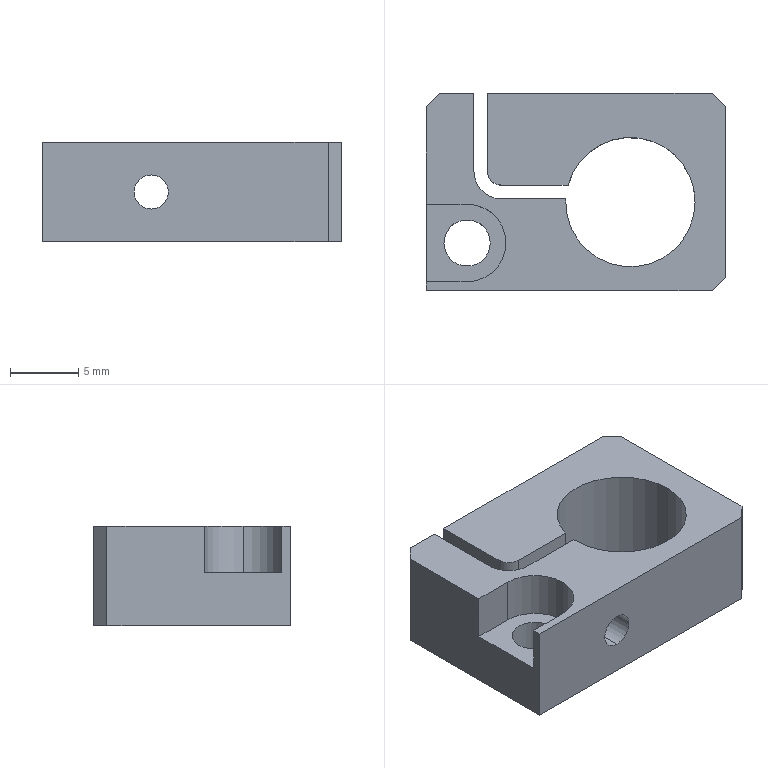Part | SolidWorks | features ICE 4, HoleWzd 3, Fillet 2, Chamfer 1, Extrusion 1 | 1 solid | 33 faces | box 22 x 14.5 x 7.3 mm | volume 1409 mm3 | plane 18 | cylinder 15 | commonest cylinder face diameters 3.4 x4 9.5 x3 2.5 x2 5.7 x2 6 x2 2 x1
STEP:
#1=CARTESIAN_POINT('',(-5.15,-3.75,3.9));
#2=VERTEX_POINT('',#1);
#3=CARTESIAN_POINT('',(-8.,-0.9,3.9));
#4=VERTEX_POINT('',#3);
#5=CARTESIAN_POINT('',(-8.,-3.75,3.9));
#6=DIRECTION('',(0.,0.,1.));
#7=DIRECTION('',(1.,0.,0.));
#8=AXIS2_PLACEMENT_3D('',#5,#6,#7);
#9=CIRCLE('',#8,2.85);
#10=EDGE_CURVE('',#2,#4,#9,.T.);
#11=ORIENTED_EDGE('',*,*,#10,.F.);
#12=CARTESIAN_POINT('',(-5.15,-3.75,7.3));
#13=VERTEX_POINT('',#12);
#14=CARTESIAN_POINT('',(-5.15,-3.75,3.9));
#15=DIRECTION('',(0.,0.,1.));
#16=VECTOR('',#15,1000.);
#17=LINE('',#14,#16);
#18=EDGE_CURVE('',#2,#13,#17,.T.);
#19=ORIENTED_EDGE('',*,*,#18,.T.);
#20=CARTESIAN_POINT('',(-8.,-0.9,7.3));
#21=VERTEX_POINT('',#20);
#22=CARTESIAN_POINT('',(-8.,-3.75,7.3));
#23=DIRECTION('',(0.,0.,1.));
#24=DIRECTION('',(1.,0.,0.));
#25=AXIS2_PLACEMENT_3D('',#22,#23,#24);
#26=CIRCLE('',#25,2.85);
#27=EDGE_CURVE('',#13,#21,#26,.T.);
#28=ORIENTED_EDGE('',*,*,#27,.T.);
#29=CARTESIAN_POINT('',(-8.,-0.9,3.9));
#30=DIRECTION('',(0.,0.,1.));
#31=VECTOR('',#30,1000.);
#32=LINE('',#29,#31);
#33=EDGE_CURVE('',#4,#21,#32,.T.);
#34=ORIENTED_EDGE('',*,*,#33,.F.);
#35=EDGE_LOOP('',(#11,#19,#28,#34));
#36=FACE_OUTER_BOUND('',#35,.T.);
#37=CARTESIAN_POINT('',(-8.,-3.75,3.9));
#38=DIRECTION('',(0.,0.,1.));
#39=DIRECTION('',(1.,0.,0.));
#40=AXIS2_PLACEMENT_3D('',#37,#38,#39);
#41=CYLINDRICAL_SURFACE('',#40,2.85);
#42=ADVANCED_FACE('',(#36),#41,.F.);
#43=CARTESIAN_POINT('',(-3.,3.85,0.65));
#44=VERTEX_POINT('',#43);
#45=CARTESIAN_POINT('',(-3.,3.85,6.65));
#46=VERTEX_POINT('',#45);
#47=CARTESIAN_POINT('',(-3.,3.85,3.65));
#48=DIRECTION('',(0.,1.,0.));
#49=DIRECTION('',(0.,0.,1.));
#50=AXIS2_PLACEMENT_3D('',#47,#48,#49);
#51=CIRCLE('',#50,3.);
#52=EDGE_CURVE('',#44,#46,#51,.T.);
#53=ORIENTED_EDGE('',*,*,#52,.F.);
#54=CARTESIAN_POINT('',(-3.,7.25,0.65));
#55=VERTEX_POINT('',#54);
#56=CARTESIAN_POINT('',(-3.,7.25,0.65));
#57=DIRECTION('',(0.,1.,0.));
#58=VECTOR('',#57,1000.);
#59=LINE('',#56,#58);
#60=EDGE_CURVE('',#44,#55,#59,.T.);
#61=ORIENTED_EDGE('',*,*,#60,.T.);
#62=CARTESIAN_POINT('',(-3.,7.25,6.65));
#63=VERTEX_POINT('',#62);
#64=CARTESIAN_POINT('',(-3.,7.25,3.65));
#65=DIRECTION('',(0.,1.,0.));
#66=DIRECTION('',(0.,0.,1.));
#67=AXIS2_PLACEMENT_3D('',#64,#65,#66);
#68=CIRCLE('',#67,3.);
#69=EDGE_CURVE('',#55,#63,#68,.T.);
#70=ORIENTED_EDGE('',*,*,#69,.T.);
#71=CARTESIAN_POINT('',(-3.,7.25,6.65));
#72=DIRECTION('',(0.,1.,0.));
#73=VECTOR('',#72,1000.);
#74=LINE('',#71,#73);
#75=EDGE_CURVE('',#46,#63,#74,.T.);
#76=ORIENTED_EDGE('',*,*,#75,.F.);
#77=EDGE_LOOP('',(#53,#61,#70,#76));
#78=FACE_OUTER_BOUND('',#77,.T.);
#79=CARTESIAN_POINT('',(-3.,7.25,3.65));
#80=DIRECTION('',(0.,1.,0.));
#81=DIRECTION('',(0.,0.,1.));
#82=AXIS2_PLACEMENT_3D('',#79,#80,#81);
#83=CYLINDRICAL_SURFACE('',#82,3.);
#84=ADVANCED_FACE('',(#78),#83,.F.);
#85=CARTESIAN_POINT('',(-3.,0.5,1.95));
#86=VERTEX_POINT('',#85);
#87=CARTESIAN_POINT('',(-3.,0.5,5.35));
#88=VERTEX_POINT('',#87);
#89=CARTESIAN_POINT('',(-3.,0.5,3.65));
#90=DIRECTION('',(0.,1.,0.));
#91=DIRECTION('',(0.,0.,1.));
#92=AXIS2_PLACEMENT_3D('',#89,#90,#91);
#93=CIRCLE('',#92,1.7);
#94=EDGE_CURVE('',#86,#88,#93,.T.);
#95=ORIENTED_EDGE('',*,*,#94,.F.);
#96=CARTESIAN_POINT('',(-3.,3.85,1.95));
#97=VERTEX_POINT('',#96);
#98=CARTESIAN_POINT('',(-3.,7.25,1.95));
#99=DIRECTION('',(0.,1.,0.));
#100=VECTOR('',#99,1000.);
#101=LINE('',#98,#100);
#102=EDGE_CURVE('',#86,#97,#101,.T.);
#103=ORIENTED_EDGE('',*,*,#102,.T.);
#104=CARTESIAN_POINT('',(-3.,3.85,5.35));
#105=VERTEX_POINT('',#104);
#106=CARTESIAN_POINT('',(-3.,3.85,3.65));
#107=DIRECTION('',(0.,1.,0.));
#108=DIRECTION('',(0.,0.,1.));
#109=AXIS2_PLACEMENT_3D('',#106,#107,#108);
#110=CIRCLE('',#109,1.7);
#111=EDGE_CURVE('',#97,#105,#110,.T.);
#112=ORIENTED_EDGE('',*,*,#111,.T.);
#113=CARTESIAN_POINT('',(-3.,7.25,5.35));
#114=DIRECTION('',(0.,1.,0.));
#115=VECTOR('',#114,1000.);
#116=LINE('',#113,#115);
#117=EDGE_CURVE('',#88,#105,#116,.T.);
#118=ORIENTED_EDGE('',*,*,#117,.F.);
#119=EDGE_LOOP('',(#95,#103,#112,#118));
#120=FACE_OUTER_BOUND('',#119,.T.);
#121=CARTESIAN_POINT('',(-3.,7.25,3.65));
#122=DIRECTION('',(0.,1.,0.));
#123=DIRECTION('',(0.,0.,1.));
#124=AXIS2_PLACEMENT_3D('',#121,#122,#123);
#125=CYLINDRICAL_SURFACE('',#124,1.7);
#126=ADVANCED_FACE('',(#120),#125,.F.);
#127=CARTESIAN_POINT('',(-3.,-7.25,2.4));
#128=VERTEX_POINT('',#127);
#129=CARTESIAN_POINT('',(-3.,-7.25,4.9));
#130=VERTEX_POINT('',#129);
#131=CARTESIAN_POINT('',(-3.,-7.25,3.65));
#132=DIRECTION('',(0.,1.,0.));
#133=DIRECTION('',(0.,0.,1.));
#134=AXIS2_PLACEMENT_3D('',#131,#132,#133);
#135=CIRCLE('',#134,1.25);
#136=EDGE_CURVE('',#128,#130,#135,.T.);
#137=ORIENTED_EDGE('',*,*,#136,.F.);
#138=CARTESIAN_POINT('',(-3.,-0.5,2.4));
#139=VERTEX_POINT('',#138);
#140=CARTESIAN_POINT('',(-3.,-0.5,2.4));
#141=DIRECTION('',(0.,1.,0.));
#142=VECTOR('',#141,1000.);
#143=LINE('',#140,#142);
#144=EDGE_CURVE('',#128,#139,#143,.T.);
#145=ORIENTED_EDGE('',*,*,#144,.T.);
#146=CARTESIAN_POINT('',(-3.,-0.5,4.9));
#147=VERTEX_POINT('',#146);
#148=CARTESIAN_POINT('',(-3.,-0.5,3.65));
#149=DIRECTION('',(0.,1.,0.));
#150=DIRECTION('',(0.,0.,1.));
#151=AXIS2_PLACEMENT_3D('',#148,#149,#150);
#152=CIRCLE('',#151,1.25);
#153=EDGE_CURVE('',#139,#147,#152,.T.);
#154=ORIENTED_EDGE('',*,*,#153,.T.);
#155=CARTESIAN_POINT('',(-3.,-0.5,4.9));
#156=DIRECTION('',(0.,1.,0.));
#157=VECTOR('',#156,1000.);
#158=LINE('',#155,#157);
#159=EDGE_CURVE('',#130,#147,#158,.T.);
#160=ORIENTED_EDGE('',*,*,#159,.F.);
#161=EDGE_LOOP('',(#137,#145,#154,#160));
#162=FACE_OUTER_BOUND('',#161,.T.);
#163=CARTESIAN_POINT('',(-3.,-0.5,3.65));
#164=DIRECTION('',(0.,1.,0.));
#165=DIRECTION('',(0.,0.,1.));
#166=AXIS2_PLACEMENT_3D('',#163,#164,#165);
#167=CYLINDRICAL_SURFACE('',#166,1.25);
#168=ADVANCED_FACE('',(#162),#167,.F.);
#169=CARTESIAN_POINT('',(-0.75,-0.75,0.));
#170=VERTEX_POINT('',#169);
#171=CARTESIAN_POINT('',(8.75,-0.75,0.));
#172=VERTEX_POINT('',#171);
#173=CARTESIAN_POINT('',(4.,-0.75,0.));
#174=DIRECTION('',(0.,0.,1.));
#175=DIRECTION('',(1.,0.,0.));
#176=AXIS2_PLACEMENT_3D('',#173,#174,#175);
#177=CIRCLE('',#176,4.75);
#178=EDGE_CURVE('',#170,#172,#177,.T.);
#179=ORIENTED_EDGE('',*,*,#178,.F.);
#180=CARTESIAN_POINT('',(-0.75,-0.75,7.3));
#181=VERTEX_POINT('',#180);
#182=CARTESIAN_POINT('',(-0.75,-0.75,0.));
#183=DIRECTION('',(0.,0.,1.));
#184=VECTOR('',#183,1000.);
#185=LINE('',#182,#184);
#186=EDGE_CURVE('',#170,#181,#185,.T.);
#187=ORIENTED_EDGE('',*,*,#186,.T.);
#188=CARTESIAN_POINT('',(8.75,-0.75,7.3));
#189=VERTEX_POINT('',#188);
#190=CARTESIAN_POINT('',(4.,-0.75,7.3));
#191=DIRECTION('',(0.,0.,1.));
#192=DIRECTION('',(1.,0.,0.));
#193=AXIS2_PLACEMENT_3D('',#190,#191,#192);
#194=CIRCLE('',#193,4.75);
#195=EDGE_CURVE('',#181,#189,#194,.T.);
#196=ORIENTED_EDGE('',*,*,#195,.T.);
#197=CARTESIAN_POINT('',(8.75,-0.75,0.));
#198=DIRECTION('',(0.,0.,1.));
#199=VECTOR('',#198,1000.);
#200=LINE('',#197,#199);
#201=EDGE_CURVE('',#172,#189,#200,.T.);
#202=ORIENTED_EDGE('',*,*,#201,.F.);
#203=EDGE_LOOP('',(#179,#187,#196,#202));
#204=FACE_OUTER_BOUND('',#203,.T.);
#205=CARTESIAN_POINT('',(4.,-0.75,0.));
#206=DIRECTION('',(0.,0.,1.));
#207=DIRECTION('',(1.,0.,0.));
#208=AXIS2_PLACEMENT_3D('',#205,#206,#207);
#209=CYLINDRICAL_SURFACE('',#208,4.75);
#210=ADVANCED_FACE('',(#204),#209,.F.);
#211=CARTESIAN_POINT('',(-0.5826,0.5,0.));
#212=VERTEX_POINT('',#211);
#213=CARTESIAN_POINT('',(4.,-0.75,0.));
#214=DIRECTION('',(0.,0.,1.));
#215=DIRECTION('',(1.,0.,0.));
#216=AXIS2_PLACEMENT_3D('',#213,#214,#215);
#217=CIRCLE('',#216,4.75);
#218=EDGE_CURVE('',#172,#212,#217,.T.);
#219=ORIENTED_EDGE('',*,*,#218,.F.);
#220=ORIENTED_EDGE('',*,*,#201,.T.);
#221=CARTESIAN_POINT('',(-0.5826,0.5,7.3));
#222=VERTEX_POINT('',#221);
#223=CARTESIAN_POINT('',(4.,-0.75,7.3));
#224=DIRECTION('',(0.,0.,1.));
#225=DIRECTION('',(1.,0.,0.));
#226=AXIS2_PLACEMENT_3D('',#223,#224,#225);
#227=CIRCLE('',#226,4.75);
#228=EDGE_CURVE('',#189,#222,#227,.T.);
#229=ORIENTED_EDGE('',*,*,#228,.T.);
#230=CARTESIAN_POINT('',(-0.5826,0.5,0.));
#231=DIRECTION('',(0.,0.,-1.));
#232=VECTOR('',#231,1000.);
#233=LINE('',#230,#232);
#234=EDGE_CURVE('',#222,#212,#233,.T.);
#235=ORIENTED_EDGE('',*,*,#234,.T.);
#236=EDGE_LOOP('',(#219,#220,#229,#235));
#237=FACE_OUTER_BOUND('',#236,.T.);
#238=CARTESIAN_POINT('',(4.,-0.75,0.));
#239=DIRECTION('',(0.,0.,1.));
#240=DIRECTION('',(1.,0.,0.));
#241=AXIS2_PLACEMENT_3D('',#238,#239,#240);
#242=CYLINDRICAL_SURFACE('',#241,4.75);
#243=ADVANCED_FACE('',(#237),#242,.F.);
#244=CARTESIAN_POINT('',(-9.7,-3.75,0.));
#245=VERTEX_POINT('',#244);
#246=CARTESIAN_POINT('',(-6.3,-3.75,0.));
#247=VERTEX_POINT('',#246);
#248=CARTESIAN_POINT('',(-8.,-3.75,0.));
#249=DIRECTION('',(0.,0.,1.));
#250=DIRECTION('',(1.,0.,0.));
#251=AXIS2_PLACEMENT_3D('',#248,#249,#250);
#252=CIRCLE('',#251,1.7);
#253=EDGE_CURVE('',#245,#247,#252,.T.);
#254=ORIENTED_EDGE('',*,*,#253,.F.);
#255=CARTESIAN_POINT('',(-9.7,-3.75,3.9));
#256=VERTEX_POINT('',#255);
#257=CARTESIAN_POINT('',(-9.7,-3.75,7.3));
#258=DIRECTION('',(0.,0.,1.));
#259=VECTOR('',#258,1000.);
#260=LINE('',#257,#259);
#261=EDGE_CURVE('',#245,#256,#260,.T.);
#262=ORIENTED_EDGE('',*,*,#261,.T.);
#263=CARTESIAN_POINT('',(-6.3,-3.75,3.9));
#264=VERTEX_POINT('',#263);
#265=CARTESIAN_POINT('',(-8.,-3.75,3.9));
#266=DIRECTION('',(0.,0.,-1.));
#267=DIRECTION('',(1.,0.,0.));
#268=AXIS2_PLACEMENT_3D('',#265,#266,#267);
#269=CIRCLE('',#268,1.7);
#270=EDGE_CURVE('',#264,#256,#269,.T.);
#271=ORIENTED_EDGE('',*,*,#270,.F.);
#272=CARTESIAN_POINT('',(-6.3,-3.75,7.3));
#273=DIRECTION('',(0.,0.,1.));
#274=VECTOR('',#273,1000.);
#275=LINE('',#272,#274);
#276=EDGE_CURVE('',#247,#264,#275,.T.);
#277=ORIENTED_EDGE('',*,*,#276,.F.);
#278=EDGE_LOOP('',(#254,#262,#271,#277));
#279=FACE_OUTER_BOUND('',#278,.T.);
#280=CARTESIAN_POINT('',(-8.,-3.75,7.3));
#281=DIRECTION('',(0.,0.,1.));
#282=DIRECTION('',(1.,0.,0.));
#283=AXIS2_PLACEMENT_3D('',#280,#281,#282);
#284=CYLINDRICAL_SURFACE('',#283,1.7);
#285=ADVANCED_FACE('',(#279),#284,.F.);
#286=ORIENTED_EDGE('',*,*,#261,.F.);
#287=CARTESIAN_POINT('',(-8.,-3.75,0.));
#288=DIRECTION('',(0.,0.,1.));
#289=DIRECTION('',(1.,0.,0.));
#290=AXIS2_PLACEMENT_3D('',#287,#288,#289);
#291=CIRCLE('',#290,1.7);
#292=EDGE_CURVE('',#247,#245,#291,.T.);
#293=ORIENTED_EDGE('',*,*,#292,.F.);
#294=ORIENTED_EDGE('',*,*,#276,.T.);
#295=CARTESIAN_POINT('',(-8.,-3.75,3.9));
#296=DIRECTION('',(0.,0.,-1.));
#297=DIRECTION('',(1.,0.,0.));
#298=AXIS2_PLACEMENT_3D('',#295,#296,#297);
#299=CIRCLE('',#298,1.7);
#300=EDGE_CURVE('',#256,#264,#299,.T.);
#301=ORIENTED_EDGE('',*,*,#300,.F.);
#302=EDGE_LOOP('',(#286,#293,#294,#301));
#303=FACE_OUTER_BOUND('',#302,.T.);
#304=CARTESIAN_POINT('',(-8.,-3.75,7.3));
#305=DIRECTION('',(0.,0.,1.));
#306=DIRECTION('',(1.,0.,0.));
#307=AXIS2_PLACEMENT_3D('',#304,#305,#306);
#308=CYLINDRICAL_SURFACE('',#307,1.7);
#309=ADVANCED_FACE('',(#303),#308,.F.);
#310=CARTESIAN_POINT('',(-7.5,7.25,0.));
#311=VERTEX_POINT('',#310);
#312=CARTESIAN_POINT('',(-10.,7.25,0.));
#313=VERTEX_POINT('',#312);
#314=CARTESIAN_POINT('',(-11.,7.25,0.));
#315=DIRECTION('',(-1.,0.,0.));
#316=VECTOR('',#315,1000.);
#317=LINE('',#314,#316);
#318=EDGE_CURVE('',#311,#313,#317,.T.);
#319=ORIENTED_EDGE('',*,*,#318,.T.);
#320=CARTESIAN_POINT('',(-10.,7.25,7.3));
#321=VERTEX_POINT('',#320);
#322=CARTESIAN_POINT('',(-10.,7.25,7.3));
#323=DIRECTION('',(0.,0.,1.));
#324=VECTOR('',#323,1000.);
#325=LINE('',#322,#324);
#326=EDGE_CURVE('',#313,#321,#325,.T.);
#327=ORIENTED_EDGE('',*,*,#326,.T.);
#328=CARTESIAN_POINT('',(-7.5,7.25,7.3));
#329=VERTEX_POINT('',#328);
#330=CARTESIAN_POINT('',(-11.,7.25,7.3));
#331=DIRECTION('',(-1.,0.,0.));
#332=VECTOR('',#331,1000.);
#333=LINE('',#330,#332);
#334=EDGE_CURVE('',#329,#321,#333,.T.);
#335=ORIENTED_EDGE('',*,*,#334,.F.);
#336=CARTESIAN_POINT('',(-7.5,7.25,-9.7));
#337=DIRECTION('',(0.,0.,1.));
#338=VECTOR('',#337,1000.);
#339=LINE('',#336,#338);
#340=EDGE_CURVE('',#311,#329,#339,.T.);
#341=ORIENTED_EDGE('',*,*,#340,.F.);
#342=EDGE_LOOP('',(#319,#327,#335,#341));
#343=FACE_OUTER_BOUND('',#342,.T.);
#344=CARTESIAN_POINT('',(-11.,7.25,7.3));
#345=DIRECTION('',(0.,-1.,0.));
#346=DIRECTION('',(0.,0.,-1.));
#347=AXIS2_PLACEMENT_3D('',#344,#345,#346);
#348=PLANE('',#347);
#349=ADVANCED_FACE('',(#343),#348,.F.);
#350=CARTESIAN_POINT('',(11.,-6.25,7.3));
#351=VERTEX_POINT('',#350);
#352=CARTESIAN_POINT('',(11.,6.25,7.3));
#353=VERTEX_POINT('',#352);
#354=CARTESIAN_POINT('',(11.,-7.25,7.3));
#355=DIRECTION('',(0.,1.,0.));
#356=VECTOR('',#355,1000.);
#357=LINE('',#354,#356);
#358=EDGE_CURVE('',#351,#353,#357,.T.);
#359=ORIENTED_EDGE('',*,*,#358,.F.);
#360=CARTESIAN_POINT('',(11.,-6.25,0.));
#361=VERTEX_POINT('',#360);
#362=CARTESIAN_POINT('',(11.,-6.25,7.3));
#363=DIRECTION('',(0.,0.,-1.));
#364=VECTOR('',#363,1000.);
#365=LINE('',#362,#364);
#366=EDGE_CURVE('',#351,#361,#365,.T.);
#367=ORIENTED_EDGE('',*,*,#366,.T.);
#368=CARTESIAN_POINT('',(11.,6.25,0.));
#369=VERTEX_POINT('',#368);
#370=CARTESIAN_POINT('',(11.,-7.25,0.));
#371=DIRECTION('',(0.,1.,0.));
#372=VECTOR('',#371,1000.);
#373=LINE('',#370,#372);
#374=EDGE_CURVE('',#361,#369,#373,.T.);
#375=ORIENTED_EDGE('',*,*,#374,.T.);
#376=CARTESIAN_POINT('',(11.,6.25,7.3));
#377=DIRECTION('',(0.,0.,1.));
#378=VECTOR('',#377,1000.);
#379=LINE('',#376,#378);
#380=EDGE_CURVE('',#369,#353,#379,.T.);
#381=ORIENTED_EDGE('',*,*,#380,.T.);
#382=EDGE_LOOP('',(#359,#367,#375,#381));
#383=FACE_OUTER_BOUND('',#382,.T.);
#384=CARTESIAN_POINT('',(11.,-7.25,7.3));
#385=DIRECTION('',(-1.,0.,0.));
#386=DIRECTION('',(0.,0.,1.));
#387=AXIS2_PLACEMENT_3D('',#384,#385,#386);
#388=PLANE('',#387);
#389=ADVANCED_FACE('',(#383),#388,.F.);
#390=CARTESIAN_POINT('',(-3.,7.25,3.65));
#391=DIRECTION('',(0.,1.,0.));
#392=DIRECTION('',(0.,0.,1.));
#393=AXIS2_PLACEMENT_3D('',#390,#391,#392);
#394=CIRCLE('',#393,3.);
#395=EDGE_CURVE('',#63,#55,#394,.T.);
#396=ORIENTED_EDGE('',*,*,#395,.F.);
#397=ORIENTED_EDGE('',*,*,#69,.F.);
#398=EDGE_LOOP('',(#396,#397));
#399=FACE_BOUND('',#398,.T.);
#400=CARTESIAN_POINT('',(10.,7.25,7.3));
#401=VERTEX_POINT('',#400);
#402=CARTESIAN_POINT('',(-6.5,7.25,7.3));
#403=VERTEX_POINT('',#402);
#404=CARTESIAN_POINT('',(-11.,7.25,7.3));
#405=DIRECTION('',(-1.,0.,0.));
#406=VECTOR('',#405,1000.);
#407=LINE('',#404,#406);
#408=EDGE_CURVE('',#401,#403,#407,.T.);
#409=ORIENTED_EDGE('',*,*,#408,.F.);
#410=CARTESIAN_POINT('',(10.,7.25,0.));
#411=VERTEX_POINT('',#410);
#412=CARTESIAN_POINT('',(10.,7.25,7.3));
#413=DIRECTION('',(0.,0.,-1.));
#414=VECTOR('',#413,1000.);
#415=LINE('',#412,#414);
#416=EDGE_CURVE('',#401,#411,#415,.T.);
#417=ORIENTED_EDGE('',*,*,#416,.T.);
#418=CARTESIAN_POINT('',(-6.5,7.25,0.));
#419=VERTEX_POINT('',#418);
#420=CARTESIAN_POINT('',(-11.,7.25,0.));
#421=DIRECTION('',(-1.,0.,0.));
#422=VECTOR('',#421,1000.);
#423=LINE('',#420,#422);
#424=EDGE_CURVE('',#411,#419,#423,.T.);
#425=ORIENTED_EDGE('',*,*,#424,.T.);
#426=CARTESIAN_POINT('',(-6.5,7.25,-9.7));
#427=DIRECTION('',(0.,0.,1.));
#428=VECTOR('',#427,1000.);
#429=LINE('',#426,#428);
#430=EDGE_CURVE('',#419,#403,#429,.T.);
#431=ORIENTED_EDGE('',*,*,#430,.T.);
#432=EDGE_LOOP('',(#409,#417,#425,#431));
#433=FACE_OUTER_BOUND('',#432,.T.);
#434=CARTESIAN_POINT('',(-11.,7.25,7.3));
#435=DIRECTION('',(0.,-1.,0.));
#436=DIRECTION('',(0.,0.,-1.));
#437=AXIS2_PLACEMENT_3D('',#434,#435,#436);
#438=PLANE('',#437);
#439=ADVANCED_FACE('',(#399,#433),#438,.F.);
#440=CARTESIAN_POINT('',(-11.,6.25,7.3));
#441=VERTEX_POINT('',#440);
#442=CARTESIAN_POINT('',(-11.,-0.9,7.3));
#443=VERTEX_POINT('',#442);
#444=CARTESIAN_POINT('',(-11.,-7.25,7.3));
#445=DIRECTION('',(0.,-1.,0.));
#446=VECTOR('',#445,1000.);
#447=LINE('',#444,#446);
#448=EDGE_CURVE('',#441,#443,#447,.T.);
#449=ORIENTED_EDGE('',*,*,#448,.F.);
#450=CARTESIAN_POINT('',(-11.,6.25,0.));
#451=VERTEX_POINT('',#450);
#452=CARTESIAN_POINT('',(-11.,6.25,7.3));
#453=DIRECTION('',(0.,0.,-1.));
#454=VECTOR('',#453,1000.);
#455=LINE('',#452,#454);
#456=EDGE_CURVE('',#441,#451,#455,.T.);
#457=ORIENTED_EDGE('',*,*,#456,.T.);
#458=CARTESIAN_POINT('',(-11.,-7.25,0.));
#459=VERTEX_POINT('',#458);
#460=CARTESIAN_POINT('',(-11.,-7.25,0.));
#461=DIRECTION('',(0.,-1.,0.));
#462=VECTOR('',#461,1000.);
#463=LINE('',#460,#462);
#464=EDGE_CURVE('',#451,#459,#463,.T.);
#465=ORIENTED_EDGE('',*,*,#464,.T.);
#466=CARTESIAN_POINT('',(-11.,-7.25,7.3));
#467=VERTEX_POINT('',#466);
#468=CARTESIAN_POINT('',(-11.,-7.25,7.3));
#469=DIRECTION('',(0.,0.,-1.));
#470=VECTOR('',#469,1000.);
#471=LINE('',#468,#470);
#472=EDGE_CURVE('',#467,#459,#471,.T.);
#473=ORIENTED_EDGE('',*,*,#472,.F.);
#474=CARTESIAN_POINT('',(-11.,-6.6,7.3));
#475=VERTEX_POINT('',#474);
#476=CARTESIAN_POINT('',(-11.,-7.25,7.3));
#477=DIRECTION('',(0.,-1.,0.));
#478=VECTOR('',#477,1000.);
#479=LINE('',#476,#478);
#480=EDGE_CURVE('',#475,#467,#479,.T.);
#481=ORIENTED_EDGE('',*,*,#480,.F.);
#482=CARTESIAN_POINT('',(-11.,-6.6,3.9));
#483=VERTEX_POINT('',#482);
#484=CARTESIAN_POINT('',(-11.,-6.6,7.3));
#485=DIRECTION('',(0.,0.,-1.));
#486=VECTOR('',#485,1000.);
#487=LINE('',#484,#486);
#488=EDGE_CURVE('',#475,#483,#487,.T.);
#489=ORIENTED_EDGE('',*,*,#488,.T.);
#490=CARTESIAN_POINT('',(-11.,-0.9,3.9));
#491=VERTEX_POINT('',#490);
#492=CARTESIAN_POINT('',(-11.,-7.25,3.9));
#493=DIRECTION('',(0.,-1.,0.));
#494=VECTOR('',#493,1000.);
#495=LINE('',#492,#494);
#496=EDGE_CURVE('',#491,#483,#495,.T.);
#497=ORIENTED_EDGE('',*,*,#496,.F.);
#498=CARTESIAN_POINT('',(-11.,-0.9,7.3));
#499=DIRECTION('',(0.,0.,1.));
#500=VECTOR('',#499,1000.);
#501=LINE('',#498,#500);
#502=EDGE_CURVE('',#491,#443,#501,.T.);
#503=ORIENTED_EDGE('',*,*,#502,.T.);
#504=EDGE_LOOP('',(#449,#457,#465,#473,#481,#489,#497,#503));
#505=FACE_OUTER_BOUND('',#504,.T.);
#506=CARTESIAN_POINT('',(-11.,-7.25,7.3));
#507=DIRECTION('',(1.,0.,0.));
#508=DIRECTION('',(0.,0.,-1.));
#509=AXIS2_PLACEMENT_3D('',#506,#507,#508);
#510=PLANE('',#509);
#511=ADVANCED_FACE('',(#505),#510,.F.);
#512=CARTESIAN_POINT('',(-3.,-7.25,3.65));
#513=DIRECTION('',(0.,1.,0.));
#514=DIRECTION('',(0.,0.,1.));
#515=AXIS2_PLACEMENT_3D('',#512,#513,#514);
#516=CIRCLE('',#515,1.25);
#517=EDGE_CURVE('',#130,#128,#516,.T.);
#518=ORIENTED_EDGE('',*,*,#517,.T.);
#519=ORIENTED_EDGE('',*,*,#136,.T.);
#520=EDGE_LOOP('',(#518,#519));
#521=FACE_BOUND('',#520,.T.);
#522=CARTESIAN_POINT('',(10.,-7.25,0.));
#523=VERTEX_POINT('',#522);
#524=CARTESIAN_POINT('',(-11.,-7.25,0.));
#525=DIRECTION('',(1.,0.,0.));
#526=VECTOR('',#525,1000.);
#527=LINE('',#524,#526);
#528=EDGE_CURVE('',#459,#523,#527,.T.);
#529=ORIENTED_EDGE('',*,*,#528,.T.);
#530=CARTESIAN_POINT('',(10.,-7.25,7.3));
#531=VERTEX_POINT('',#530);
#532=CARTESIAN_POINT('',(10.,-7.25,7.3));
#533=DIRECTION('',(0.,0.,1.));
#534=VECTOR('',#533,1000.);
#535=LINE('',#532,#534);
#536=EDGE_CURVE('',#523,#531,#535,.T.);
#537=ORIENTED_EDGE('',*,*,#536,.T.);
#538=CARTESIAN_POINT('',(-11.,-7.25,7.3));
#539=DIRECTION('',(1.,0.,0.));
#540=VECTOR('',#539,1000.);
#541=LINE('',#538,#540);
#542=EDGE_CURVE('',#467,#531,#541,.T.);
#543=ORIENTED_EDGE('',*,*,#542,.F.);
#544=ORIENTED_EDGE('',*,*,#472,.T.);
#545=EDGE_LOOP('',(#529,#537,#543,#544));
#546=FACE_OUTER_BOUND('',#545,.T.);
#547=CARTESIAN_POINT('',(-11.,-7.25,7.3));
#548=DIRECTION('',(0.,1.,0.));
#549=DIRECTION('',(0.,0.,1.));
#550=AXIS2_PLACEMENT_3D('',#547,#548,#549);
#551=PLANE('',#550);
#552=ADVANCED_FACE('',(#521,#546),#551,.F.);
#553=ORIENTED_EDGE('',*,*,#542,.T.);
#554=CARTESIAN_POINT('',(11.,-6.25,7.3));
#555=DIRECTION('',(0.7071,0.7071,0.));
#556=VECTOR('',#555,1000.);
#557=LINE('',#554,#556);
#558=EDGE_CURVE('',#531,#351,#557,.T.);
#559=ORIENTED_EDGE('',*,*,#558,.T.);
#560=ORIENTED_EDGE('',*,*,#358,.T.);
#561=CARTESIAN_POINT('',(10.,7.25,7.3));
#562=DIRECTION('',(-0.7071,0.7071,0.));
#563=VECTOR('',#562,1000.);
#564=LINE('',#561,#563);
#565=EDGE_CURVE('',#353,#401,#564,.T.);
#566=ORIENTED_EDGE('',*,*,#565,.T.);
#567=ORIENTED_EDGE('',*,*,#408,.T.);
#568=CARTESIAN_POINT('',(-6.5,1.5,7.3));
#569=VERTEX_POINT('',#568);
#570=CARTESIAN_POINT('',(-6.5,0.5,7.3));
#571=DIRECTION('',(0.,1.,0.));
#572=VECTOR('',#571,1000.);
#573=LINE('',#570,#572);
#574=EDGE_CURVE('',#569,#403,#573,.T.);
#575=ORIENTED_EDGE('',*,*,#574,.F.);
#576=CARTESIAN_POINT('',(-5.5,0.5,7.3));
#577=VERTEX_POINT('',#576);
#578=CARTESIAN_POINT('',(-5.5,1.5,7.3));
#579=DIRECTION('',(0.,0.,1.));
#580=DIRECTION('',(-1.,0.,0.));
#581=AXIS2_PLACEMENT_3D('',#578,#579,#580);
#582=CIRCLE('',#581,1.);
#583=EDGE_CURVE('',#569,#577,#582,.T.);
#584=ORIENTED_EDGE('',*,*,#583,.T.);
#585=CARTESIAN_POINT('',(7.5,0.5,7.3));
#586=DIRECTION('',(-1.,0.,0.));
#587=VECTOR('',#586,1000.);
#588=LINE('',#585,#587);
#589=EDGE_CURVE('',#222,#577,#588,.T.);
#590=ORIENTED_EDGE('',*,*,#589,.F.);
#591=ORIENTED_EDGE('',*,*,#228,.F.);
#592=ORIENTED_EDGE('',*,*,#195,.F.);
#593=CARTESIAN_POINT('',(-0.7434,-0.5,7.3));
#594=VERTEX_POINT('',#593);
#595=CARTESIAN_POINT('',(4.,-0.75,7.3));
#596=DIRECTION('',(0.,0.,1.));
#597=DIRECTION('',(1.,0.,0.));
#598=AXIS2_PLACEMENT_3D('',#595,#596,#597);
#599=CIRCLE('',#598,4.75);
#600=EDGE_CURVE('',#594,#181,#599,.T.);
#601=ORIENTED_EDGE('',*,*,#600,.F.);
#602=CARTESIAN_POINT('',(-5.5,-0.5,7.3));
#603=VERTEX_POINT('',#602);
#604=CARTESIAN_POINT('',(7.5,-0.5,7.3));
#605=DIRECTION('',(1.,0.,0.));
#606=VECTOR('',#605,1000.);
#607=LINE('',#604,#606);
#608=EDGE_CURVE('',#603,#594,#607,.T.);
#609=ORIENTED_EDGE('',*,*,#608,.F.);
#610=CARTESIAN_POINT('',(-7.5,1.5,7.3));
#611=VERTEX_POINT('',#610);
#612=CARTESIAN_POINT('',(-5.5,1.5,7.3));
#613=DIRECTION('',(0.,0.,-1.));
#614=DIRECTION('',(-1.,0.,0.));
#615=AXIS2_PLACEMENT_3D('',#612,#613,#614);
#616=CIRCLE('',#615,2.);
#617=EDGE_CURVE('',#603,#611,#616,.T.);
#618=ORIENTED_EDGE('',*,*,#617,.T.);
#619=CARTESIAN_POINT('',(-7.5,-0.5,7.3));
#620=DIRECTION('',(0.,-1.,0.));
#621=VECTOR('',#620,1000.);
#622=LINE('',#619,#621);
#623=EDGE_CURVE('',#329,#611,#622,.T.);
#624=ORIENTED_EDGE('',*,*,#623,.F.);
#625=ORIENTED_EDGE('',*,*,#334,.T.);
#626=CARTESIAN_POINT('',(-11.,6.25,7.3));
#627=DIRECTION('',(-0.7071,-0.7071,0.));
#628=VECTOR('',#627,1000.);
#629=LINE('',#626,#628);
#630=EDGE_CURVE('',#321,#441,#629,.T.);
#631=ORIENTED_EDGE('',*,*,#630,.T.);
#632=ORIENTED_EDGE('',*,*,#448,.T.);
#633=CARTESIAN_POINT('',(-8.,-0.9,7.3));
#634=DIRECTION('',(-1.,0.,0.));
#635=VECTOR('',#634,1000.);
#636=LINE('',#633,#635);
#637=EDGE_CURVE('',#21,#443,#636,.T.);
#638=ORIENTED_EDGE('',*,*,#637,.F.);
#639=ORIENTED_EDGE('',*,*,#27,.F.);
#640=CARTESIAN_POINT('',(-8.,-6.6,7.3));
#641=VERTEX_POINT('',#640);
#642=CARTESIAN_POINT('',(-8.,-3.75,7.3));
#643=DIRECTION('',(0.,0.,1.));
#644=DIRECTION('',(1.,0.,0.));
#645=AXIS2_PLACEMENT_3D('',#642,#643,#644);
#646=CIRCLE('',#645,2.85);
#647=EDGE_CURVE('',#641,#13,#646,.T.);
#648=ORIENTED_EDGE('',*,*,#647,.F.);
#649=CARTESIAN_POINT('',(-8.,-6.6,7.3));
#650=DIRECTION('',(1.,0.,0.));
#651=VECTOR('',#650,1000.);
#652=LINE('',#649,#651);
#653=EDGE_CURVE('',#475,#641,#652,.T.);
#654=ORIENTED_EDGE('',*,*,#653,.F.);
#655=ORIENTED_EDGE('',*,*,#480,.T.);
#656=EDGE_LOOP('',(#553,#559,#560,#566,#567,#575,#584,#590,#591,#592,#601,#609,#618,#624,#625,#631,#632,#638,#639,#648,#654,#655));
#657=FACE_OUTER_BOUND('',#656,.T.);
#658=CARTESIAN_POINT('',(0.,0.,7.3));
#659=DIRECTION('',(0.,0.,-1.));
#660=DIRECTION('',(-1.,0.,0.));
#661=AXIS2_PLACEMENT_3D('',#658,#659,#660);
#662=PLANE('',#661);
#663=ADVANCED_FACE('',(#657),#662,.F.);
#664=ORIENTED_EDGE('',*,*,#374,.F.);
#665=CARTESIAN_POINT('',(8.625,-8.625,0.));
#666=DIRECTION('',(-0.7071,-0.7071,0.));
#667=VECTOR('',#666,1000.);
#668=LINE('',#665,#667);
#669=EDGE_CURVE('',#361,#523,#668,.T.);
#670=ORIENTED_EDGE('',*,*,#669,.T.);
#671=ORIENTED_EDGE('',*,*,#528,.F.);
#672=ORIENTED_EDGE('',*,*,#464,.F.);
#673=CARTESIAN_POINT('',(-8.625,8.625,0.));
#674=DIRECTION('',(0.7071,0.7071,0.));
#675=VECTOR('',#674,1000.);
#676=LINE('',#673,#675);
#677=EDGE_CURVE('',#451,#313,#676,.T.);
#678=ORIENTED_EDGE('',*,*,#677,.T.);
#679=ORIENTED_EDGE('',*,*,#318,.F.);
#680=CARTESIAN_POINT('',(-7.5,1.5,0.));
#681=VERTEX_POINT('',#680);
#682=CARTESIAN_POINT('',(-7.5,-0.5,0.));
#683=DIRECTION('',(0.,-1.,0.));
#684=VECTOR('',#683,1000.);
#685=LINE('',#682,#684);
#686=EDGE_CURVE('',#311,#681,#685,.T.);
#687=ORIENTED_EDGE('',*,*,#686,.T.);
#688=CARTESIAN_POINT('',(-5.5,-0.5,0.));
#689=VERTEX_POINT('',#688);
#690=CARTESIAN_POINT('',(-5.5,1.5,0.));
#691=DIRECTION('',(0.,0.,1.));
#692=DIRECTION('',(-1.,0.,0.));
#693=AXIS2_PLACEMENT_3D('',#690,#691,#692);
#694=CIRCLE('',#693,2.);
#695=EDGE_CURVE('',#681,#689,#694,.T.);
#696=ORIENTED_EDGE('',*,*,#695,.T.);
#697=CARTESIAN_POINT('',(-0.7434,-0.5,0.));
#698=VERTEX_POINT('',#697);
#699=CARTESIAN_POINT('',(7.5,-0.5,0.));
#700=DIRECTION('',(1.,0.,0.));
#701=VECTOR('',#700,1000.);
#702=LINE('',#699,#701);
#703=EDGE_CURVE('',#689,#698,#702,.T.);
#704=ORIENTED_EDGE('',*,*,#703,.T.);
#705=CARTESIAN_POINT('',(4.,-0.75,0.));
#706=DIRECTION('',(0.,0.,1.));
#707=DIRECTION('',(1.,0.,0.));
#708=AXIS2_PLACEMENT_3D('',#705,#706,#707);
#709=CIRCLE('',#708,4.75);
#710=EDGE_CURVE('',#698,#170,#709,.T.);
#711=ORIENTED_EDGE('',*,*,#710,.T.);
#712=ORIENTED_EDGE('',*,*,#178,.T.);
#713=ORIENTED_EDGE('',*,*,#218,.T.);
#714=CARTESIAN_POINT('',(-5.5,0.5,0.));
#715=VERTEX_POINT('',#714);
#716=CARTESIAN_POINT('',(7.5,0.5,0.));
#717=DIRECTION('',(-1.,0.,0.));
#718=VECTOR('',#717,1000.);
#719=LINE('',#716,#718);
#720=EDGE_CURVE('',#212,#715,#719,.T.);
#721=ORIENTED_EDGE('',*,*,#720,.T.);
#722=CARTESIAN_POINT('',(-6.5,1.5,0.));
#723=VERTEX_POINT('',#722);
#724=CARTESIAN_POINT('',(-5.5,1.5,0.));
#725=DIRECTION('',(0.,0.,-1.));
#726=DIRECTION('',(-1.,0.,0.));
#727=AXIS2_PLACEMENT_3D('',#724,#725,#726);
#728=CIRCLE('',#727,1.);
#729=EDGE_CURVE('',#715,#723,#728,.T.);
#730=ORIENTED_EDGE('',*,*,#729,.T.);
#731=CARTESIAN_POINT('',(-6.5,0.,0.));
#732=DIRECTION('',(0.,-1.,0.));
#733=VECTOR('',#732,1000.);
#734=LINE('',#731,#733);
#735=EDGE_CURVE('',#419,#723,#734,.T.);
#736=ORIENTED_EDGE('',*,*,#735,.F.);
#737=ORIENTED_EDGE('',*,*,#424,.F.);
#738=CARTESIAN_POINT('',(8.625,8.625,0.));
#739=DIRECTION('',(0.7071,-0.7071,0.));
#740=VECTOR('',#739,1000.);
#741=LINE('',#738,#740);
#742=EDGE_CURVE('',#411,#369,#741,.T.);
#743=ORIENTED_EDGE('',*,*,#742,.T.);
#744=EDGE_LOOP('',(#664,#670,#671,#672,#678,#679,#687,#696,#704,#711,#712,#713,#721,#730,#736,#737,#743));
#745=FACE_OUTER_BOUND('',#744,.T.);
#746=ORIENTED_EDGE('',*,*,#292,.T.);
#747=ORIENTED_EDGE('',*,*,#253,.T.);
#748=EDGE_LOOP('',(#746,#747));
#749=FACE_BOUND('',#748,.T.);
#750=CARTESIAN_POINT('',(0.,0.,0.));
#751=DIRECTION('',(0.,0.,-1.));
#752=DIRECTION('',(-1.,0.,0.));
#753=AXIS2_PLACEMENT_3D('',#750,#751,#752);
#754=PLANE('',#753);
#755=ADVANCED_FACE('',(#745,#749),#754,.T.);
#756=ORIENTED_EDGE('',*,*,#186,.F.);
#757=ORIENTED_EDGE('',*,*,#710,.F.);
#758=CARTESIAN_POINT('',(-0.7434,-0.5,0.));
#759=DIRECTION('',(0.,0.,1.));
#760=VECTOR('',#759,1000.);
#761=LINE('',#758,#760);
#762=EDGE_CURVE('',#698,#594,#761,.T.);
#763=ORIENTED_EDGE('',*,*,#762,.T.);
#764=ORIENTED_EDGE('',*,*,#600,.T.);
#765=EDGE_LOOP('',(#756,#757,#763,#764));
#766=FACE_OUTER_BOUND('',#765,.T.);
#767=CARTESIAN_POINT('',(4.,-0.75,0.));
#768=DIRECTION('',(0.,0.,1.));
#769=DIRECTION('',(1.,0.,0.));
#770=AXIS2_PLACEMENT_3D('',#767,#768,#769);
#771=CYLINDRICAL_SURFACE('',#770,4.75);
#772=ADVANCED_FACE('',(#766),#771,.F.);
#773=CARTESIAN_POINT('',(-3.,0.5,3.65));
#774=DIRECTION('',(0.,1.,0.));
#775=DIRECTION('',(0.,0.,1.));
#776=AXIS2_PLACEMENT_3D('',#773,#774,#775);
#777=CIRCLE('',#776,1.7);
#778=EDGE_CURVE('',#88,#86,#777,.T.);
#779=ORIENTED_EDGE('',*,*,#778,.T.);
#780=ORIENTED_EDGE('',*,*,#94,.T.);
#781=EDGE_LOOP('',(#779,#780));
#782=FACE_BOUND('',#781,.T.);
#783=ORIENTED_EDGE('',*,*,#589,.T.);
#784=CARTESIAN_POINT('',(-5.5,0.5,0.));
#785=DIRECTION('',(0.,0.,-1.));
#786=VECTOR('',#785,1000.);
#787=LINE('',#784,#786);
#788=EDGE_CURVE('',#577,#715,#787,.T.);
#789=ORIENTED_EDGE('',*,*,#788,.T.);
#790=ORIENTED_EDGE('',*,*,#720,.F.);
#791=ORIENTED_EDGE('',*,*,#234,.F.);
#792=EDGE_LOOP('',(#783,#789,#790,#791));
#793=FACE_OUTER_BOUND('',#792,.T.);
#794=CARTESIAN_POINT('',(7.5,0.5,0.));
#795=DIRECTION('',(0.,1.,0.));
#796=DIRECTION('',(0.,0.,1.));
#797=AXIS2_PLACEMENT_3D('',#794,#795,#796);
#798=PLANE('',#797);
#799=ADVANCED_FACE('',(#782,#793),#798,.F.);
#800=ORIENTED_EDGE('',*,*,#703,.F.);
#801=CARTESIAN_POINT('',(-5.5,-0.5,7.3));
#802=DIRECTION('',(0.,0.,1.));
#803=VECTOR('',#802,1000.);
#804=LINE('',#801,#803);
#805=EDGE_CURVE('',#689,#603,#804,.T.);
#806=ORIENTED_EDGE('',*,*,#805,.T.);
#807=ORIENTED_EDGE('',*,*,#608,.T.);
#808=ORIENTED_EDGE('',*,*,#762,.F.);
#809=EDGE_LOOP('',(#800,#806,#807,#808));
#810=FACE_OUTER_BOUND('',#809,.T.);
#811=CARTESIAN_POINT('',(-3.,-0.5,3.65));
#812=DIRECTION('',(0.,1.,0.));
#813=DIRECTION('',(0.,0.,1.));
#814=AXIS2_PLACEMENT_3D('',#811,#812,#813);
#815=CIRCLE('',#814,1.25);
#816=EDGE_CURVE('',#147,#139,#815,.T.);
#817=ORIENTED_EDGE('',*,*,#816,.F.);
#818=ORIENTED_EDGE('',*,*,#153,.F.);
#819=EDGE_LOOP('',(#817,#818));
#820=FACE_BOUND('',#819,.T.);
#821=CARTESIAN_POINT('',(7.5,-0.5,0.));
#822=DIRECTION('',(0.,-1.,0.));
#823=DIRECTION('',(0.,0.,-1.));
#824=AXIS2_PLACEMENT_3D('',#821,#822,#823);
#825=PLANE('',#824);
#826=ADVANCED_FACE('',(#810,#820),#825,.F.);
#827=ORIENTED_EDGE('',*,*,#623,.T.);
#828=CARTESIAN_POINT('',(-7.5,1.5,0.));
#829=DIRECTION('',(0.,0.,-1.));
#830=VECTOR('',#829,1000.);
#831=LINE('',#828,#830);
#832=EDGE_CURVE('',#611,#681,#831,.T.);
#833=ORIENTED_EDGE('',*,*,#832,.T.);
#834=ORIENTED_EDGE('',*,*,#686,.F.);
#835=ORIENTED_EDGE('',*,*,#340,.T.);
#836=EDGE_LOOP('',(#827,#833,#834,#835));
#837=FACE_OUTER_BOUND('',#836,.T.);
#838=CARTESIAN_POINT('',(-7.5,-0.5,0.));
#839=DIRECTION('',(-1.,0.,0.));
#840=DIRECTION('',(0.,0.,1.));
#841=AXIS2_PLACEMENT_3D('',#838,#839,#840);
#842=PLANE('',#841);
#843=ADVANCED_FACE('',(#837),#842,.F.);
#844=ORIENTED_EDGE('',*,*,#735,.T.);
#845=CARTESIAN_POINT('',(-6.5,1.5,-9.7));
#846=DIRECTION('',(0.,0.,1.));
#847=VECTOR('',#846,1000.);
#848=LINE('',#845,#847);
#849=EDGE_CURVE('',#723,#569,#848,.T.);
#850=ORIENTED_EDGE('',*,*,#849,.T.);
#851=ORIENTED_EDGE('',*,*,#574,.T.);
#852=ORIENTED_EDGE('',*,*,#430,.F.);
#853=EDGE_LOOP('',(#844,#850,#851,#852));
#854=FACE_OUTER_BOUND('',#853,.T.);
#855=CARTESIAN_POINT('',(-6.5,0.5,-9.7));
#856=DIRECTION('',(1.,0.,0.));
#857=DIRECTION('',(0.,0.,-1.));
#858=AXIS2_PLACEMENT_3D('',#855,#856,#857);
#859=PLANE('',#858);
#860=ADVANCED_FACE('',(#854),#859,.F.);
#861=ORIENTED_EDGE('',*,*,#695,.F.);
#862=ORIENTED_EDGE('',*,*,#832,.F.);
#863=ORIENTED_EDGE('',*,*,#617,.F.);
#864=ORIENTED_EDGE('',*,*,#805,.F.);
#865=EDGE_LOOP('',(#861,#862,#863,#864));
#866=FACE_OUTER_BOUND('',#865,.T.);
#867=CARTESIAN_POINT('',(-5.5,1.5,0.));
#868=DIRECTION('',(0.,0.,-1.));
#869=DIRECTION('',(-1.,0.,0.));
#870=AXIS2_PLACEMENT_3D('',#867,#868,#869);
#871=CYLINDRICAL_SURFACE('',#870,2.);
#872=ADVANCED_FACE('',(#866),#871,.F.);
#873=ORIENTED_EDGE('',*,*,#729,.F.);
#874=ORIENTED_EDGE('',*,*,#788,.F.);
#875=ORIENTED_EDGE('',*,*,#583,.F.);
#876=ORIENTED_EDGE('',*,*,#849,.F.);
#877=EDGE_LOOP('',(#873,#874,#875,#876));
#878=FACE_OUTER_BOUND('',#877,.T.);
#879=CARTESIAN_POINT('',(-5.5,1.5,-9.7));
#880=DIRECTION('',(0.,0.,1.));
#881=DIRECTION('',(1.,0.,0.));
#882=AXIS2_PLACEMENT_3D('',#879,#880,#881);
#883=CYLINDRICAL_SURFACE('',#882,1.);
#884=ADVANCED_FACE('',(#878),#883,.T.);
#885=ORIENTED_EDGE('',*,*,#144,.F.);
#886=ORIENTED_EDGE('',*,*,#517,.F.);
#887=ORIENTED_EDGE('',*,*,#159,.T.);
#888=ORIENTED_EDGE('',*,*,#816,.T.);
#889=EDGE_LOOP('',(#885,#886,#887,#888));
#890=FACE_OUTER_BOUND('',#889,.T.);
#891=CARTESIAN_POINT('',(-3.,-0.5,3.65));
#892=DIRECTION('',(0.,1.,0.));
#893=DIRECTION('',(0.,0.,1.));
#894=AXIS2_PLACEMENT_3D('',#891,#892,#893);
#895=CYLINDRICAL_SURFACE('',#894,1.25);
#896=ADVANCED_FACE('',(#890),#895,.F.);
#897=ORIENTED_EDGE('',*,*,#102,.F.);
#898=ORIENTED_EDGE('',*,*,#778,.F.);
#899=ORIENTED_EDGE('',*,*,#117,.T.);
#900=CARTESIAN_POINT('',(-3.,3.85,3.65));
#901=DIRECTION('',(0.,1.,0.));
#902=DIRECTION('',(0.,0.,1.));
#903=AXIS2_PLACEMENT_3D('',#900,#901,#902);
#904=CIRCLE('',#903,1.7);
#905=EDGE_CURVE('',#105,#97,#904,.T.);
#906=ORIENTED_EDGE('',*,*,#905,.T.);
#907=EDGE_LOOP('',(#897,#898,#899,#906));
#908=FACE_OUTER_BOUND('',#907,.T.);
#909=CARTESIAN_POINT('',(-3.,7.25,3.65));
#910=DIRECTION('',(0.,1.,0.));
#911=DIRECTION('',(0.,0.,1.));
#912=AXIS2_PLACEMENT_3D('',#909,#910,#911);
#913=CYLINDRICAL_SURFACE('',#912,1.7);
#914=ADVANCED_FACE('',(#908),#913,.F.);
#915=ORIENTED_EDGE('',*,*,#905,.F.);
#916=ORIENTED_EDGE('',*,*,#111,.F.);
#917=EDGE_LOOP('',(#915,#916));
#918=FACE_BOUND('',#917,.T.);
#919=CARTESIAN_POINT('',(-3.,3.85,3.65));
#920=DIRECTION('',(0.,1.,0.));
#921=DIRECTION('',(0.,0.,1.));
#922=AXIS2_PLACEMENT_3D('',#919,#920,#921);
#923=CIRCLE('',#922,3.);
#924=EDGE_CURVE('',#46,#44,#923,.T.);
#925=ORIENTED_EDGE('',*,*,#924,.T.);
#926=ORIENTED_EDGE('',*,*,#52,.T.);
#927=EDGE_LOOP('',(#925,#926));
#928=FACE_OUTER_BOUND('',#927,.T.);
#929=CARTESIAN_POINT('',(-1.3,3.85,3.65));
#930=DIRECTION('',(0.,-1.,0.));
#931=DIRECTION('',(0.,0.,-1.));
#932=AXIS2_PLACEMENT_3D('',#929,#930,#931);
#933=PLANE('',#932);
#934=ADVANCED_FACE('',(#918,#928),#933,.F.);
#935=ORIENTED_EDGE('',*,*,#60,.F.);
#936=ORIENTED_EDGE('',*,*,#924,.F.);
#937=ORIENTED_EDGE('',*,*,#75,.T.);
#938=ORIENTED_EDGE('',*,*,#395,.T.);
#939=EDGE_LOOP('',(#935,#936,#937,#938));
#940=FACE_OUTER_BOUND('',#939,.T.);
#941=CARTESIAN_POINT('',(-3.,7.25,3.65));
#942=DIRECTION('',(0.,1.,0.));
#943=DIRECTION('',(0.,0.,1.));
#944=AXIS2_PLACEMENT_3D('',#941,#942,#943);
#945=CYLINDRICAL_SURFACE('',#944,3.);
#946=ADVANCED_FACE('',(#940),#945,.F.);
#947=ORIENTED_EDGE('',*,*,#653,.T.);
#948=CARTESIAN_POINT('',(-8.,-6.6,3.9));
#949=VERTEX_POINT('',#948);
#950=CARTESIAN_POINT('',(-8.,-6.6,3.9));
#951=DIRECTION('',(0.,0.,1.));
#952=VECTOR('',#951,1000.);
#953=LINE('',#950,#952);
#954=EDGE_CURVE('',#949,#641,#953,.T.);
#955=ORIENTED_EDGE('',*,*,#954,.F.);
#956=CARTESIAN_POINT('',(-8.,-6.6,3.9));
#957=DIRECTION('',(1.,0.,0.));
#958=VECTOR('',#957,1000.);
#959=LINE('',#956,#958);
#960=EDGE_CURVE('',#483,#949,#959,.T.);
#961=ORIENTED_EDGE('',*,*,#960,.F.);
#962=ORIENTED_EDGE('',*,*,#488,.F.);
#963=EDGE_LOOP('',(#947,#955,#961,#962));
#964=FACE_OUTER_BOUND('',#963,.T.);
#965=CARTESIAN_POINT('',(-8.,-6.6,3.9));
#966=DIRECTION('',(0.,-1.,0.));
#967=DIRECTION('',(0.,0.,-1.));
#968=AXIS2_PLACEMENT_3D('',#965,#966,#967);
#969=PLANE('',#968);
#970=ADVANCED_FACE('',(#964),#969,.F.);
#971=CARTESIAN_POINT('',(-8.,-0.9,3.9));
#972=DIRECTION('',(-1.,0.,0.));
#973=VECTOR('',#972,1000.);
#974=LINE('',#971,#973);
#975=EDGE_CURVE('',#4,#491,#974,.T.);
#976=ORIENTED_EDGE('',*,*,#975,.F.);
#977=ORIENTED_EDGE('',*,*,#33,.T.);
#978=ORIENTED_EDGE('',*,*,#637,.T.);
#979=ORIENTED_EDGE('',*,*,#502,.F.);
#980=EDGE_LOOP('',(#976,#977,#978,#979));
#981=FACE_OUTER_BOUND('',#980,.T.);
#982=CARTESIAN_POINT('',(-8.,-0.9,3.9));
#983=DIRECTION('',(0.,1.,0.));
#984=DIRECTION('',(-1.,0.,0.));
#985=AXIS2_PLACEMENT_3D('',#982,#983,#984);
#986=PLANE('',#985);
#987=ADVANCED_FACE('',(#981),#986,.F.);
#988=ORIENTED_EDGE('',*,*,#270,.T.);
#989=ORIENTED_EDGE('',*,*,#300,.T.);
#990=EDGE_LOOP('',(#988,#989));
#991=FACE_BOUND('',#990,.T.);
#992=ORIENTED_EDGE('',*,*,#496,.T.);
#993=ORIENTED_EDGE('',*,*,#960,.T.);
#994=CARTESIAN_POINT('',(-8.,-3.75,3.9));
#995=DIRECTION('',(0.,0.,1.));
#996=DIRECTION('',(1.,0.,0.));
#997=AXIS2_PLACEMENT_3D('',#994,#995,#996);
#998=CIRCLE('',#997,2.85);
#999=EDGE_CURVE('',#949,#2,#998,.T.);
#1000=ORIENTED_EDGE('',*,*,#999,.T.);
#1001=ORIENTED_EDGE('',*,*,#10,.T.);
#1002=ORIENTED_EDGE('',*,*,#975,.T.);
#1003=EDGE_LOOP('',(#992,#993,#1000,#1001,#1002));
#1004=FACE_OUTER_BOUND('',#1003,.T.);
#1005=CARTESIAN_POINT('',(-8.,-3.75,3.9));
#1006=DIRECTION('',(0.,0.,1.));
#1007=DIRECTION('',(1.,0.,0.));
#1008=AXIS2_PLACEMENT_3D('',#1005,#1006,#1007);
#1009=PLANE('',#1008);
#1010=ADVANCED_FACE('',(#991,#1004),#1009,.T.);
#1011=ORIENTED_EDGE('',*,*,#18,.F.);
#1012=ORIENTED_EDGE('',*,*,#999,.F.);
#1013=ORIENTED_EDGE('',*,*,#954,.T.);
#1014=ORIENTED_EDGE('',*,*,#647,.T.);
#1015=EDGE_LOOP('',(#1011,#1012,#1013,#1014));
#1016=FACE_OUTER_BOUND('',#1015,.T.);
#1017=CARTESIAN_POINT('',(-8.,-3.75,3.9));
#1018=DIRECTION('',(0.,0.,1.));
#1019=DIRECTION('',(1.,0.,0.));
#1020=AXIS2_PLACEMENT_3D('',#1017,#1018,#1019);
#1021=CYLINDRICAL_SURFACE('',#1020,2.85);
#1022=ADVANCED_FACE('',(#1016),#1021,.F.);
#1023=ORIENTED_EDGE('',*,*,#558,.F.);
#1024=ORIENTED_EDGE('',*,*,#536,.F.);
#1025=ORIENTED_EDGE('',*,*,#669,.F.);
#1026=ORIENTED_EDGE('',*,*,#366,.F.);
#1027=EDGE_LOOP('',(#1023,#1024,#1025,#1026));
#1028=FACE_OUTER_BOUND('',#1027,.T.);
#1029=CARTESIAN_POINT('',(11.,-6.25,7.3));
#1030=DIRECTION('',(-0.7071,0.7071,0.));
#1031=DIRECTION('',(0.,0.,-1.));
#1032=AXIS2_PLACEMENT_3D('',#1029,#1030,#1031);
#1033=PLANE('',#1032);
#1034=ADVANCED_FACE('',(#1028),#1033,.F.);
#1035=ORIENTED_EDGE('',*,*,#565,.F.);
#1036=ORIENTED_EDGE('',*,*,#380,.F.);
#1037=ORIENTED_EDGE('',*,*,#742,.F.);
#1038=ORIENTED_EDGE('',*,*,#416,.F.);
#1039=EDGE_LOOP('',(#1035,#1036,#1037,#1038));
#1040=FACE_OUTER_BOUND('',#1039,.T.);
#1041=CARTESIAN_POINT('',(10.,7.25,7.3));
#1042=DIRECTION('',(-0.7071,-0.7071,0.));
#1043=DIRECTION('',(0.,0.,-1.));
#1044=AXIS2_PLACEMENT_3D('',#1041,#1042,#1043);
#1045=PLANE('',#1044);
#1046=ADVANCED_FACE('',(#1040),#1045,.F.);
#1047=ORIENTED_EDGE('',*,*,#630,.F.);
#1048=ORIENTED_EDGE('',*,*,#326,.F.);
#1049=ORIENTED_EDGE('',*,*,#677,.F.);
#1050=ORIENTED_EDGE('',*,*,#456,.F.);
#1051=EDGE_LOOP('',(#1047,#1048,#1049,#1050));
#1052=FACE_OUTER_BOUND('',#1051,.T.);
#1053=CARTESIAN_POINT('',(-11.,6.25,7.3));
#1054=DIRECTION('',(0.7071,-0.7071,0.));
#1055=DIRECTION('',(0.,0.,-1.));
#1056=AXIS2_PLACEMENT_3D('',#1053,#1054,#1055);
#1057=PLANE('',#1056);
#1058=ADVANCED_FACE('',(#1052),#1057,.F.);
#1059=CLOSED_SHELL('',(#42,#84,#126,#168,#210,#243,#285,#309,#349,#389,#439,#511,#552,#663,#755,#772,#799,#826,#843,#860,#872,#884,#896,#914,#934,#946,#970,#987,#1010,#1022,#1034,#1046,#1058));
#1060=MANIFOLD_SOLID_BREP('',#1059);
#1061=CARTESIAN_POINT('',(0.,0.,0.));
#1062=DIRECTION('',(0.,0.,1.));
#1063=DIRECTION('',(1.,0.,0.));
#1064=AXIS2_PLACEMENT_3D('',#1061,#1062,#1063);
#1065=(LENGTH_UNIT()NAMED_UNIT(*)SI_UNIT(.MILLI.,.METRE.));
#1066=UNCERTAINTY_MEASURE_WITH_UNIT(LENGTH_MEASURE(0.00001),#1065,'','');
#1067=(NAMED_UNIT(*)PLANE_ANGLE_UNIT()SI_UNIT($,.RADIAN.));
#1068=(NAMED_UNIT(*)SI_UNIT($,.STERADIAN.)SOLID_ANGLE_UNIT());
#1069=(GEOMETRIC_REPRESENTATION_CONTEXT(3)GLOBAL_UNCERTAINTY_ASSIGNED_CONTEXT((#1066))GLOBAL_UNIT_ASSIGNED_CONTEXT((#1065,#1067,#1068))REPRESENTATION_CONTEXT('',''));
#1070=ADVANCED_BREP_SHAPE_REPRESENTATION('',(#1060,#1064),#1069);